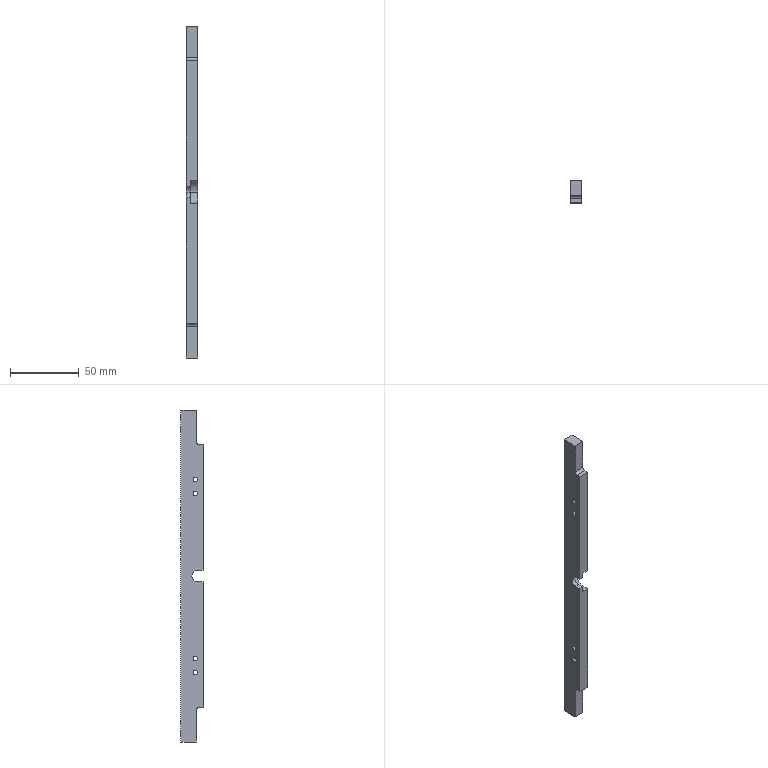Part | SolidWorks | features HoleWzd 2, ICE 2, Cut 1, Extrusion 1 | 1 solid | 58 faces | box 8 x 16 x 241 mm | volume 26977 mm3 | cylinder 30 | plane 20 | cone 8 | commonest cylinder face diameters 3.3 x8 3.4 x8 6 x8 4 x2 8.2 x2 16 x2